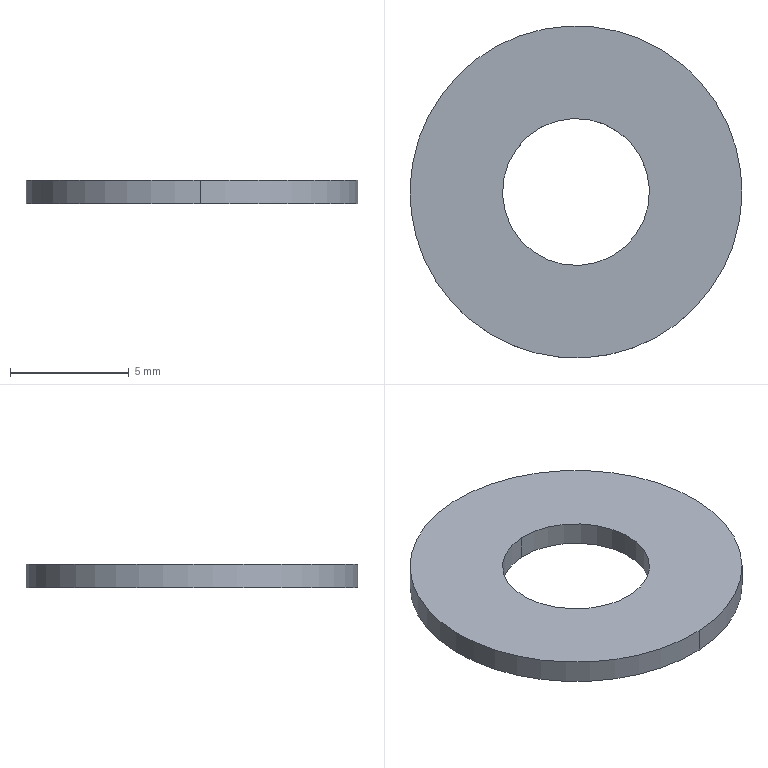Part | SolidWorks | features BaseBody 1 | 1 solid | 6 faces | box 14 x 14 x 1 mm | volume 123.747 mm3 | cylinder 4 | plane 2 | commonest cylinder face diameters 6.2 x2 14 x2
STEP:
#1=CARTESIAN_POINT('',(404.946,41.096,61.7));
#2=VERTEX_POINT('',#1);
#3=CARTESIAN_POINT('',(405.254,34.904,61.7));
#4=VERTEX_POINT('',#3);
#5=CARTESIAN_POINT('',(405.1,38.,61.7));
#6=DIRECTION('',(0.,0.,-1.));
#7=DIRECTION('',(0.04954,-0.9988,0.));
#8=AXIS2_PLACEMENT_3D('',#5,#6,#7);
#9=CIRCLE('',#8,3.1);
#10=EDGE_CURVE('',#2,#4,#9,.T.);
#11=ORIENTED_EDGE('',*,*,#10,.T.);
#12=CARTESIAN_POINT('',(405.254,34.904,62.7));
#13=VERTEX_POINT('',#12);
#14=CARTESIAN_POINT('',(405.254,34.904,61.7));
#15=DIRECTION('',(0.,0.,1.));
#16=VECTOR('',#15,1000.);
#17=LINE('',#14,#16);
#18=EDGE_CURVE('',#4,#13,#17,.T.);
#19=ORIENTED_EDGE('',*,*,#18,.T.);
#20=CARTESIAN_POINT('',(404.946,41.096,62.7));
#21=VERTEX_POINT('',#20);
#22=CARTESIAN_POINT('',(405.1,38.,62.7));
#23=DIRECTION('',(0.,0.,-1.));
#24=DIRECTION('',(0.04954,-0.9988,0.));
#25=AXIS2_PLACEMENT_3D('',#22,#23,#24);
#26=CIRCLE('',#25,3.1);
#27=EDGE_CURVE('',#21,#13,#26,.T.);
#28=ORIENTED_EDGE('',*,*,#27,.F.);
#29=CARTESIAN_POINT('',(404.946,41.096,61.7));
#30=DIRECTION('',(0.,0.,1.));
#31=VECTOR('',#30,1000.);
#32=LINE('',#29,#31);
#33=EDGE_CURVE('',#2,#21,#32,.T.);
#34=ORIENTED_EDGE('',*,*,#33,.F.);
#35=EDGE_LOOP('',(#11,#19,#28,#34));
#36=FACE_OUTER_BOUND('',#35,.T.);
#37=CARTESIAN_POINT('',(405.1,38.,61.7));
#38=DIRECTION('',(0.,0.,1.));
#39=DIRECTION('',(-0.04954,0.9988,0.));
#40=AXIS2_PLACEMENT_3D('',#37,#38,#39);
#41=CYLINDRICAL_SURFACE('',#40,3.1);
#42=ADVANCED_FACE('',(#36),#41,.F.);
#43=CARTESIAN_POINT('',(405.447,31.009,61.7));
#44=VERTEX_POINT('',#43);
#45=CARTESIAN_POINT('',(404.753,44.991,61.7));
#46=VERTEX_POINT('',#45);
#47=CARTESIAN_POINT('',(405.1,38.,61.7));
#48=DIRECTION('',(0.,0.,-1.));
#49=DIRECTION('',(0.04954,-0.9988,0.));
#50=AXIS2_PLACEMENT_3D('',#47,#48,#49);
#51=CIRCLE('',#50,7.);
#52=EDGE_CURVE('',#44,#46,#51,.T.);
#53=ORIENTED_EDGE('',*,*,#52,.F.);
#54=CARTESIAN_POINT('',(405.447,31.009,62.7));
#55=VERTEX_POINT('',#54);
#56=CARTESIAN_POINT('',(405.447,31.009,61.7));
#57=DIRECTION('',(0.,0.,1.));
#58=VECTOR('',#57,1000.);
#59=LINE('',#56,#58);
#60=EDGE_CURVE('',#44,#55,#59,.T.);
#61=ORIENTED_EDGE('',*,*,#60,.T.);
#62=CARTESIAN_POINT('',(404.753,44.991,62.7));
#63=VERTEX_POINT('',#62);
#64=CARTESIAN_POINT('',(405.1,38.,62.7));
#65=DIRECTION('',(0.,0.,-1.));
#66=DIRECTION('',(0.04954,-0.9988,0.));
#67=AXIS2_PLACEMENT_3D('',#64,#65,#66);
#68=CIRCLE('',#67,7.);
#69=EDGE_CURVE('',#55,#63,#68,.T.);
#70=ORIENTED_EDGE('',*,*,#69,.T.);
#71=CARTESIAN_POINT('',(404.753,44.991,61.7));
#72=DIRECTION('',(0.,0.,1.));
#73=VECTOR('',#72,1000.);
#74=LINE('',#71,#73);
#75=EDGE_CURVE('',#46,#63,#74,.T.);
#76=ORIENTED_EDGE('',*,*,#75,.F.);
#77=EDGE_LOOP('',(#53,#61,#70,#76));
#78=FACE_OUTER_BOUND('',#77,.T.);
#79=CARTESIAN_POINT('',(405.1,38.,61.7));
#80=DIRECTION('',(0.,0.,1.));
#81=DIRECTION('',(-0.04954,0.9988,0.));
#82=AXIS2_PLACEMENT_3D('',#79,#80,#81);
#83=CYLINDRICAL_SURFACE('',#82,7.);
#84=ADVANCED_FACE('',(#78),#83,.T.);
#85=CARTESIAN_POINT('',(405.1,38.,61.7));
#86=DIRECTION('',(0.,0.,-1.));
#87=DIRECTION('',(0.04954,-0.9988,0.));
#88=AXIS2_PLACEMENT_3D('',#85,#86,#87);
#89=CIRCLE('',#88,7.);
#90=EDGE_CURVE('',#46,#44,#89,.T.);
#91=ORIENTED_EDGE('',*,*,#90,.T.);
#92=ORIENTED_EDGE('',*,*,#52,.T.);
#93=EDGE_LOOP('',(#91,#92));
#94=FACE_OUTER_BOUND('',#93,.T.);
#95=ORIENTED_EDGE('',*,*,#10,.F.);
#96=CARTESIAN_POINT('',(405.1,38.,61.7));
#97=DIRECTION('',(0.,0.,-1.));
#98=DIRECTION('',(0.04954,-0.9988,0.));
#99=AXIS2_PLACEMENT_3D('',#96,#97,#98);
#100=CIRCLE('',#99,3.1);
#101=EDGE_CURVE('',#4,#2,#100,.T.);
#102=ORIENTED_EDGE('',*,*,#101,.F.);
#103=EDGE_LOOP('',(#95,#102));
#104=FACE_BOUND('',#103,.T.);
#105=CARTESIAN_POINT('',(405.1,38.,61.7));
#106=DIRECTION('',(0.,0.,-1.));
#107=DIRECTION('',(0.04954,-0.9988,0.));
#108=AXIS2_PLACEMENT_3D('',#105,#106,#107);
#109=PLANE('',#108);
#110=ADVANCED_FACE('',(#94,#104),#109,.T.);
#111=CARTESIAN_POINT('',(405.1,38.,62.7));
#112=DIRECTION('',(0.,0.,-1.));
#113=DIRECTION('',(0.04954,-0.9988,0.));
#114=AXIS2_PLACEMENT_3D('',#111,#112,#113);
#115=CIRCLE('',#114,7.);
#116=EDGE_CURVE('',#63,#55,#115,.T.);
#117=ORIENTED_EDGE('',*,*,#116,.F.);
#118=ORIENTED_EDGE('',*,*,#69,.F.);
#119=EDGE_LOOP('',(#117,#118));
#120=FACE_OUTER_BOUND('',#119,.T.);
#121=ORIENTED_EDGE('',*,*,#27,.T.);
#122=CARTESIAN_POINT('',(405.1,38.,62.7));
#123=DIRECTION('',(0.,0.,-1.));
#124=DIRECTION('',(0.04954,-0.9988,0.));
#125=AXIS2_PLACEMENT_3D('',#122,#123,#124);
#126=CIRCLE('',#125,3.1);
#127=EDGE_CURVE('',#13,#21,#126,.T.);
#128=ORIENTED_EDGE('',*,*,#127,.T.);
#129=EDGE_LOOP('',(#121,#128));
#130=FACE_BOUND('',#129,.T.);
#131=CARTESIAN_POINT('',(405.1,38.,62.7));
#132=DIRECTION('',(0.,0.,-1.));
#133=DIRECTION('',(0.04954,-0.9988,0.));
#134=AXIS2_PLACEMENT_3D('',#131,#132,#133);
#135=PLANE('',#134);
#136=ADVANCED_FACE('',(#120,#130),#135,.F.);
#137=ORIENTED_EDGE('',*,*,#60,.F.);
#138=ORIENTED_EDGE('',*,*,#90,.F.);
#139=ORIENTED_EDGE('',*,*,#75,.T.);
#140=ORIENTED_EDGE('',*,*,#116,.T.);
#141=EDGE_LOOP('',(#137,#138,#139,#140));
#142=FACE_OUTER_BOUND('',#141,.T.);
#143=CARTESIAN_POINT('',(405.1,38.,61.7));
#144=DIRECTION('',(0.,0.,1.));
#145=DIRECTION('',(-0.04954,0.9988,0.));
#146=AXIS2_PLACEMENT_3D('',#143,#144,#145);
#147=CYLINDRICAL_SURFACE('',#146,7.);
#148=ADVANCED_FACE('',(#142),#147,.T.);
#149=ORIENTED_EDGE('',*,*,#18,.F.);
#150=ORIENTED_EDGE('',*,*,#101,.T.);
#151=ORIENTED_EDGE('',*,*,#33,.T.);
#152=ORIENTED_EDGE('',*,*,#127,.F.);
#153=EDGE_LOOP('',(#149,#150,#151,#152));
#154=FACE_OUTER_BOUND('',#153,.T.);
#155=CARTESIAN_POINT('',(405.1,38.,61.7));
#156=DIRECTION('',(0.,0.,1.));
#157=DIRECTION('',(-0.04954,0.9988,0.));
#158=AXIS2_PLACEMENT_3D('',#155,#156,#157);
#159=CYLINDRICAL_SURFACE('',#158,3.1);
#160=ADVANCED_FACE('',(#154),#159,.F.);
#161=CLOSED_SHELL('',(#42,#84,#110,#136,#148,#160));
#162=MANIFOLD_SOLID_BREP('',#161);
#163=CARTESIAN_POINT('',(0.,0.,0.));
#164=DIRECTION('',(0.,0.,1.));
#165=DIRECTION('',(1.,0.,0.));
#166=AXIS2_PLACEMENT_3D('',#163,#164,#165);
#167=(LENGTH_UNIT()NAMED_UNIT(*)SI_UNIT(.MILLI.,.METRE.));
#168=UNCERTAINTY_MEASURE_WITH_UNIT(LENGTH_MEASURE(0.00001),#167,'','');
#169=(NAMED_UNIT(*)PLANE_ANGLE_UNIT()SI_UNIT($,.RADIAN.));
#170=(NAMED_UNIT(*)SI_UNIT($,.STERADIAN.)SOLID_ANGLE_UNIT());
#171=(GEOMETRIC_REPRESENTATION_CONTEXT(3)GLOBAL_UNCERTAINTY_ASSIGNED_CONTEXT((#168))GLOBAL_UNIT_ASSIGNED_CONTEXT((#167,#169,#170))REPRESENTATION_CONTEXT('',''));
#172=ADVANCED_BREP_SHAPE_REPRESENTATION('',(#162,#166),#171);